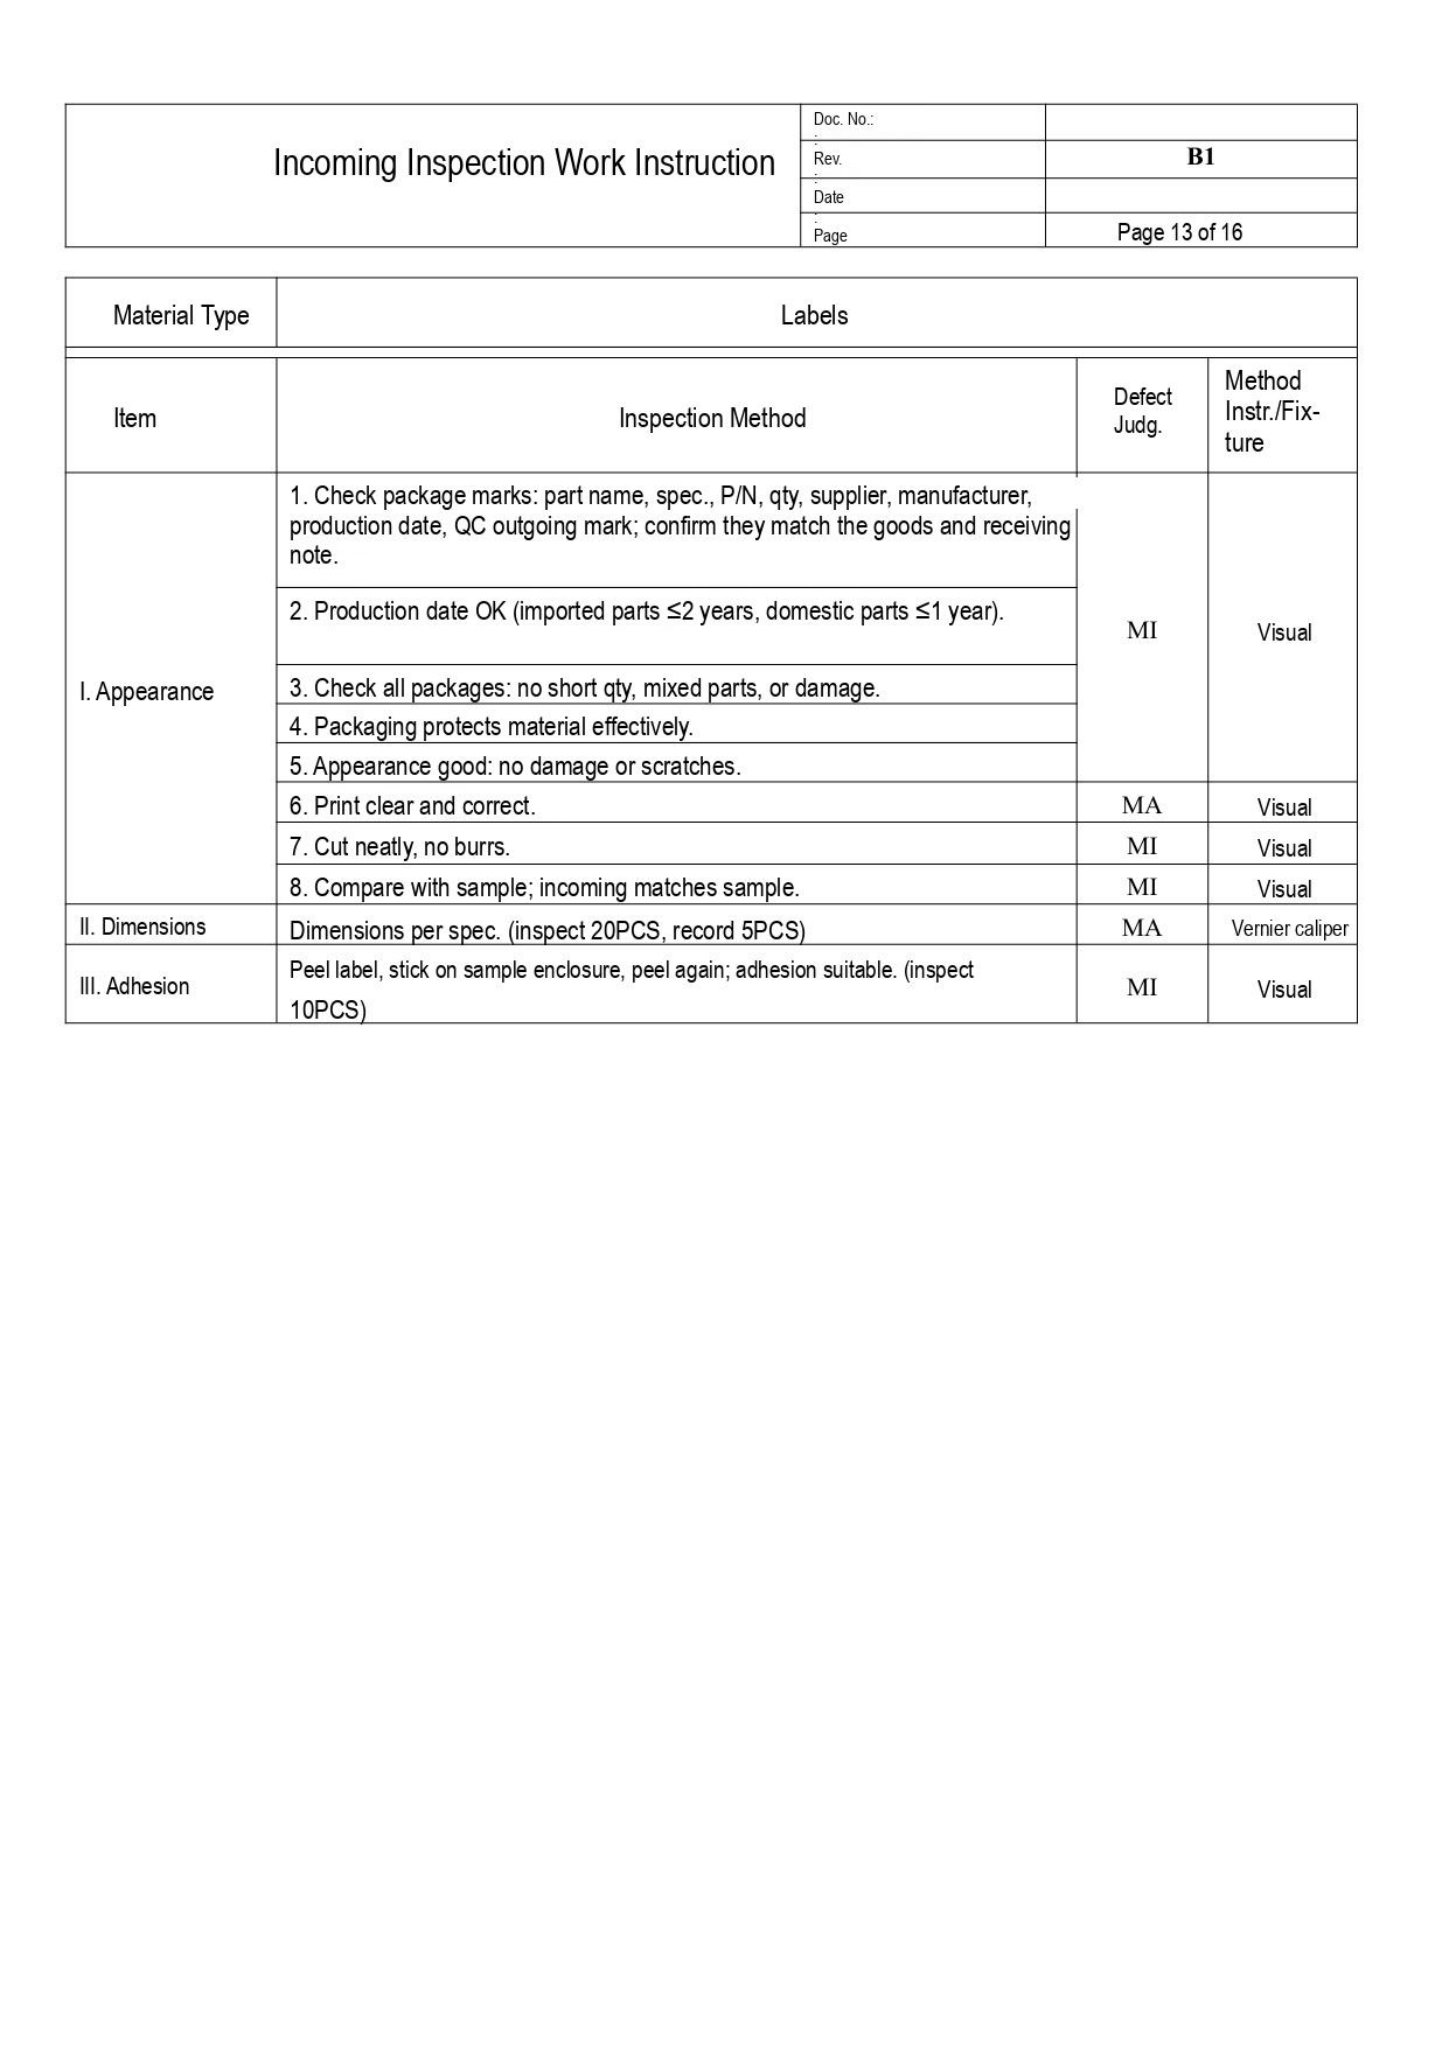| Incoming Inspection Work Instruction | Doc. No.: | |
|---|---|---|
| | Rev. | B1 |
| | Date | |
| | Page | Page 13 of 16 |

| Material Type | Labels | | |
|---|---|---|---|
| Item | Inspection Method | Defect Judg. | Method Instr./Fix-ture |
| I. Appearance | 1. Check package marks: part name, spec., P/N, qty, supplier, manufacturer, production date, QC outgoing mark; confirm they match the goods and receiving note. | MI | Visual |
| | 2. Production date OK (imported parts ≤2 years, domestic parts ≤1 year). | | |
| | 3. Check all packages: no short qty, mixed parts, or damage. | | |
| | 4. Packaging protects material effectively. | | |
| | 5. Appearance good: no damage or scratches. | | |
| | 6. Print clear and correct. | MA | Visual |
| | 7. Cut neatly, no burrs. | MI | Visual |
| | 8. Compare with sample; incoming matches sample. | MI | Visual |
| II. Dimensions | Dimensions per spec. (inspect 20PCS, record 5PCS) | MA | Vernier caliper |
| III. Adhesion | Peel label, stick on sample enclosure, peel again; adhesion suitable. (inspect 10PCS) | MI | Visual |
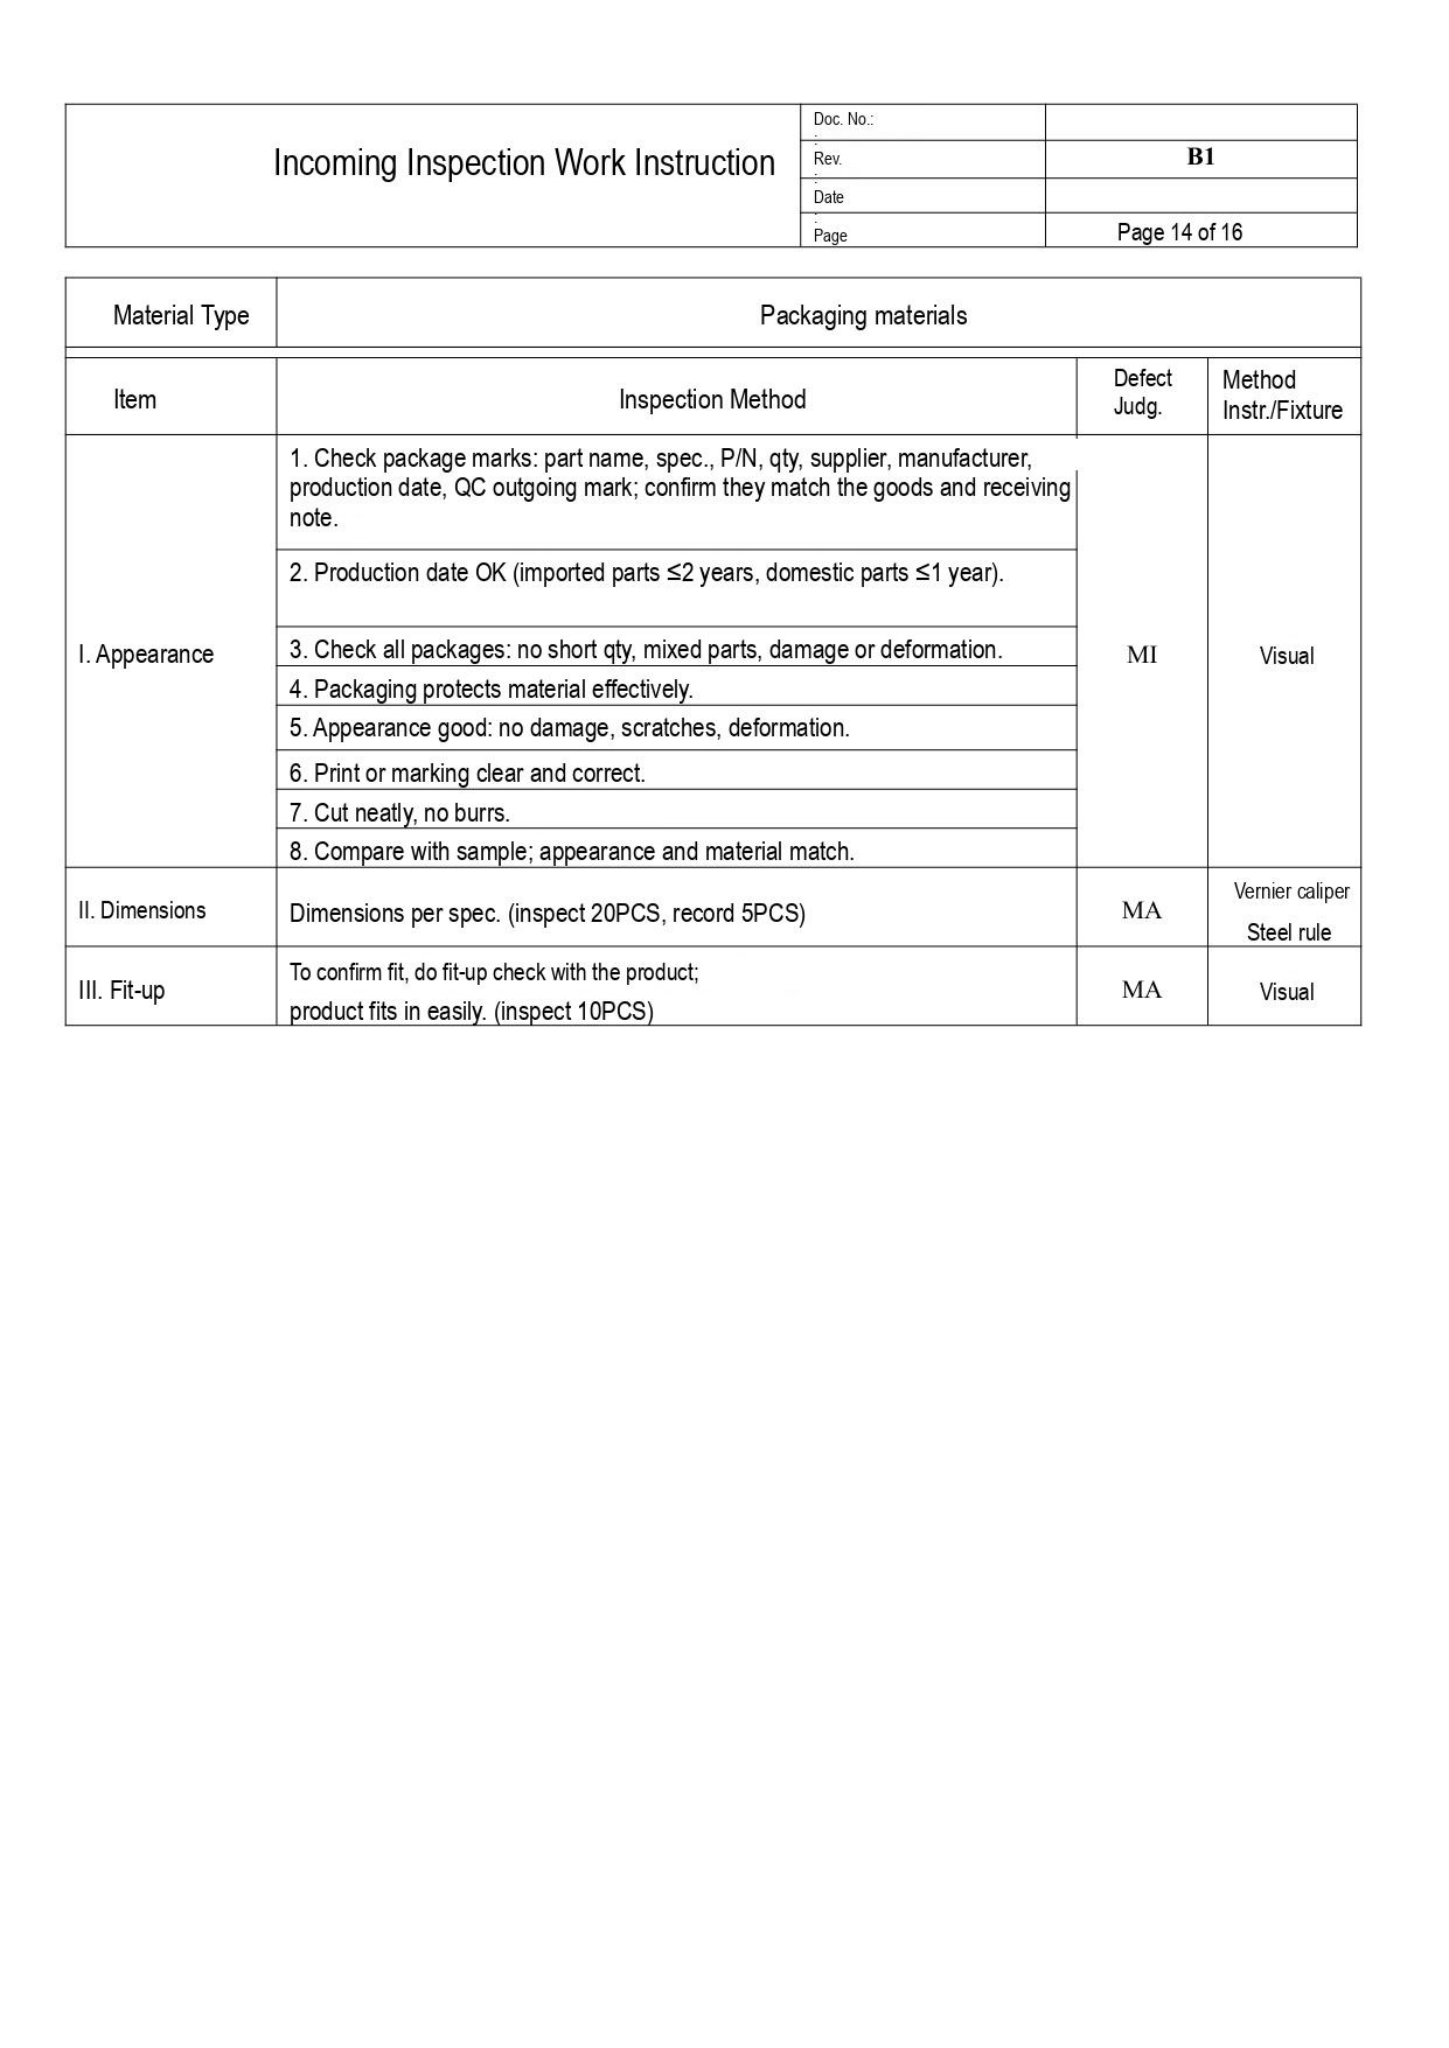| Incoming Inspection Work Instruction | Doc. No.: | |
|---|---|---|
| | Rev. | B1 |
| | Date | |
| | Page | Page 14 of 16 |

| Material Type | Packaging materials | | |
|---|---|---|---|
| Item | Inspection Method | Defect Judg. | Method Instr./Fixture |
| I. Appearance | 1. Check package marks: part name, spec., P/N, qty, supplier, manufacturer, production date, QC outgoing mark; confirm they match the goods and receiving note. | MI | Visual |
| | 2. Production date OK (imported parts ≤2 years, domestic parts ≤1 year). | | |
| | 3. Check all packages: no short qty, mixed parts, damage or deformation. | | |
| | 4. Packaging protects material effectively. | | |
| | 5. Appearance good: no damage, scratches, deformation. | | |
| | 6. Print or marking clear and correct. | | |
| | 7. Cut neatly, no burrs. | | |
| | 8. Compare with sample; appearance and material match. | | |
| II. Dimensions | Dimensions per spec. (inspect 20PCS, record 5PCS) | MA | Vernier caliper<br>Steel rule |
| III. Fit-up | To confirm fit, do fit-up check with the product;<br>product fits in easily. (inspect 10PCS) | MA | Visual |
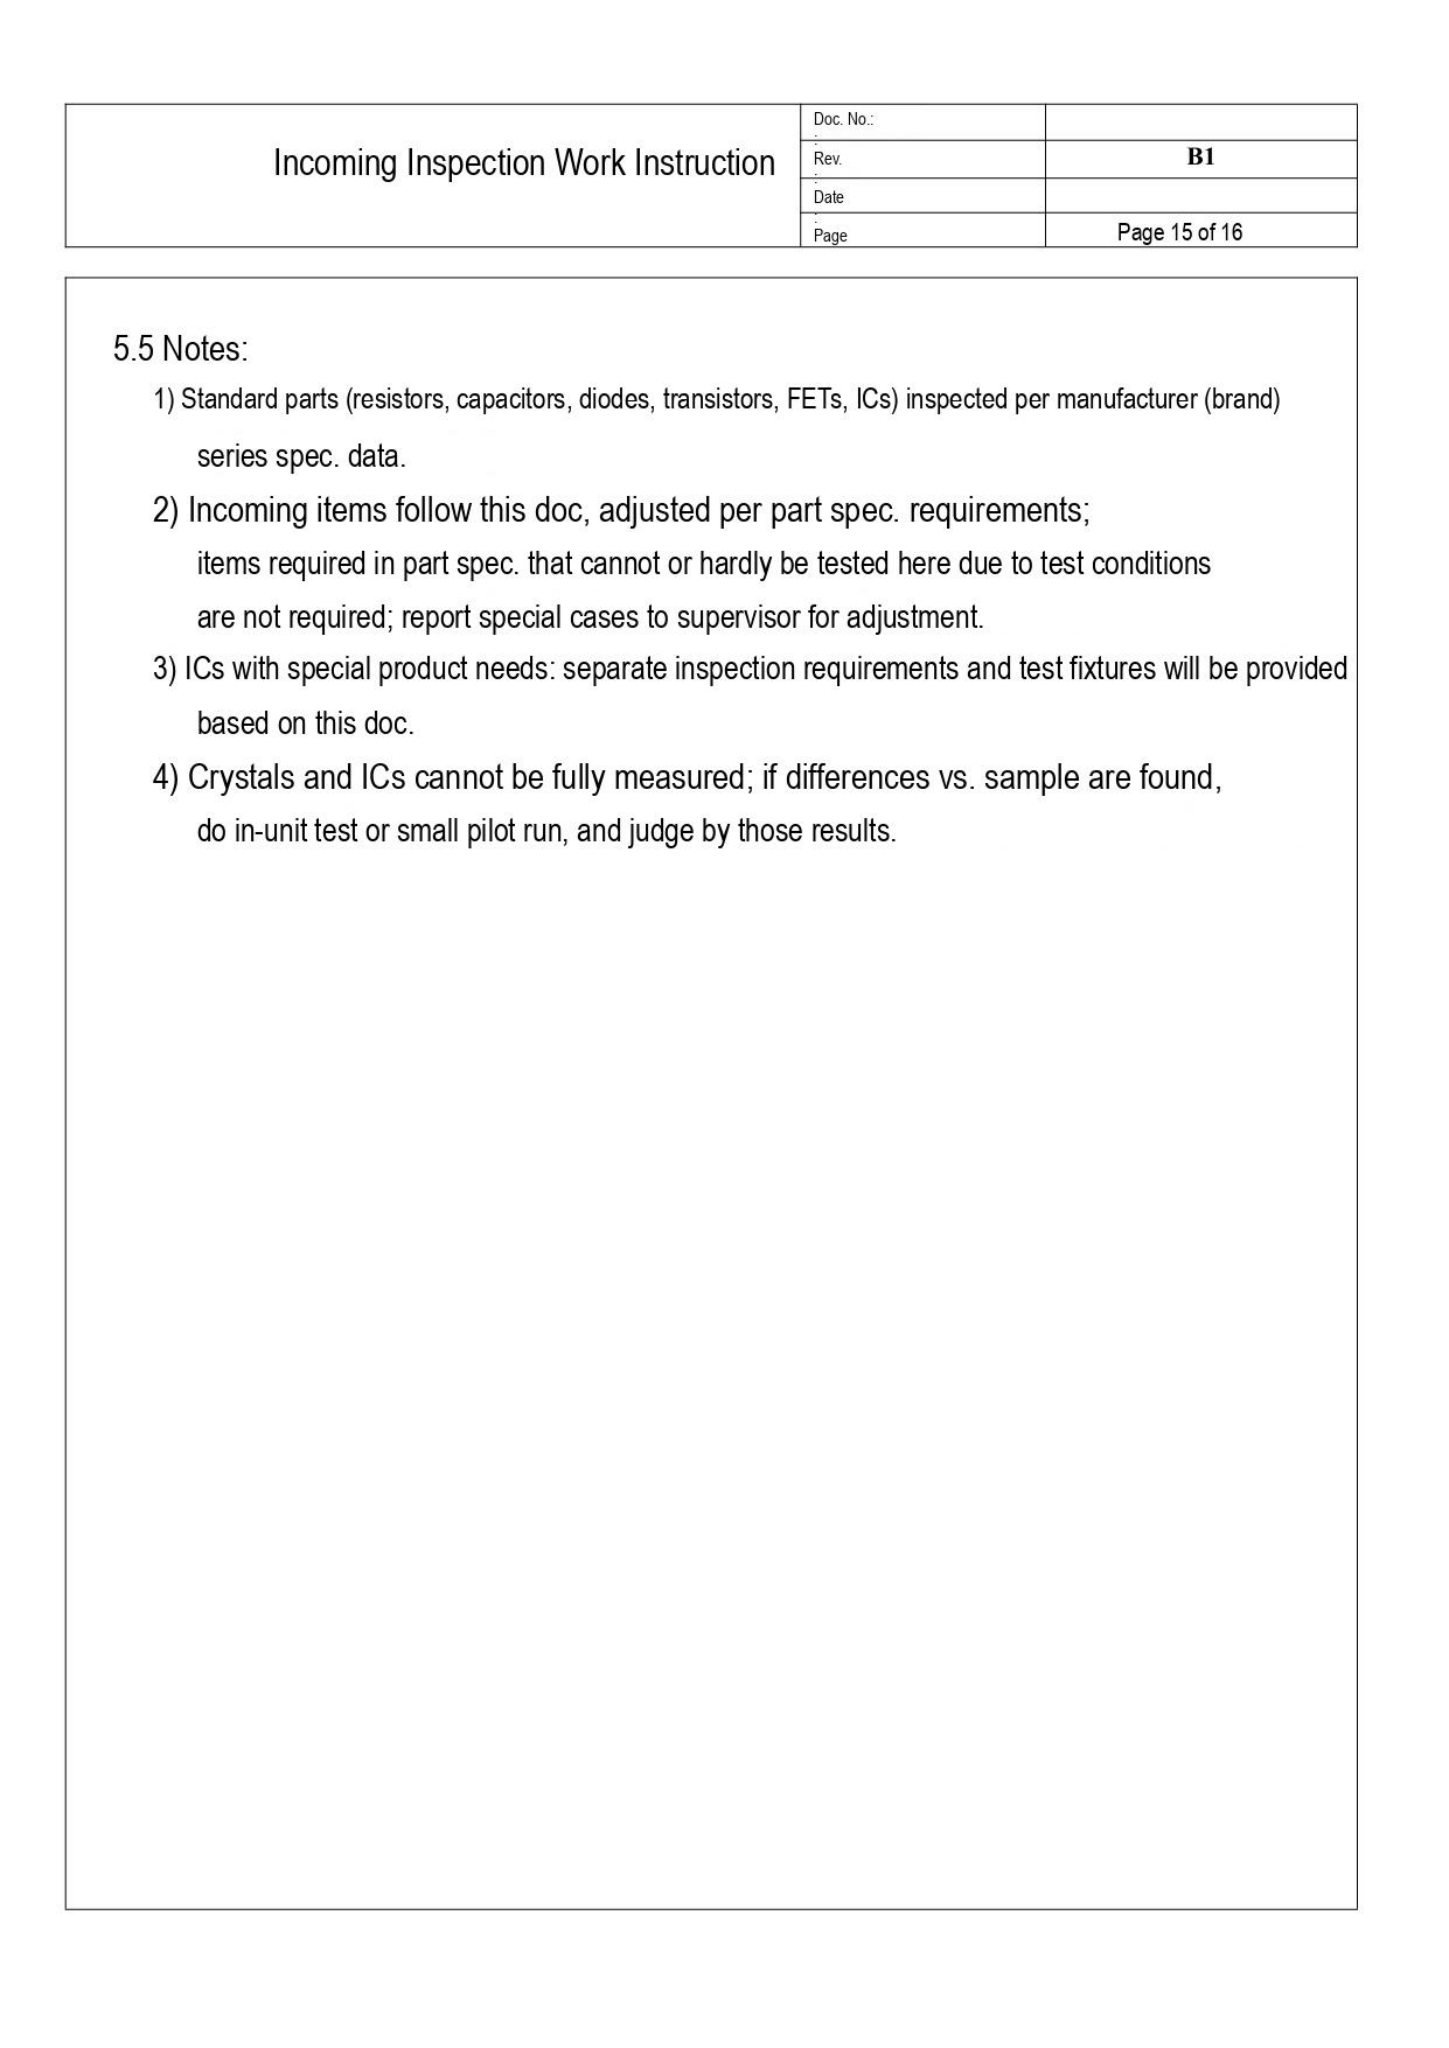Incoming Inspection Work Instruction

| | |
|---|---|
| Doc. No.: | |
| Rev. | B1 |
| Date | |
| Page | Page 15 of 16 |

5.5 Notes:

1) Standard parts (resistors, capacitors, diodes, transistors, FETs, ICs) inspected per manufacturer (brand) series spec. data.

2) Incoming items follow this doc, adjusted per part spec. requirements; items required in part spec. that cannot or hardly be tested here due to test conditions are not required; report special cases to supervisor for adjustment.

3) ICs with special product needs: separate inspection requirements and test fixtures will be provided based on this doc.

4) Crystals and ICs cannot be fully measured; if differences vs. sample are found, do in-unit test or small pilot run, and judge by those results.